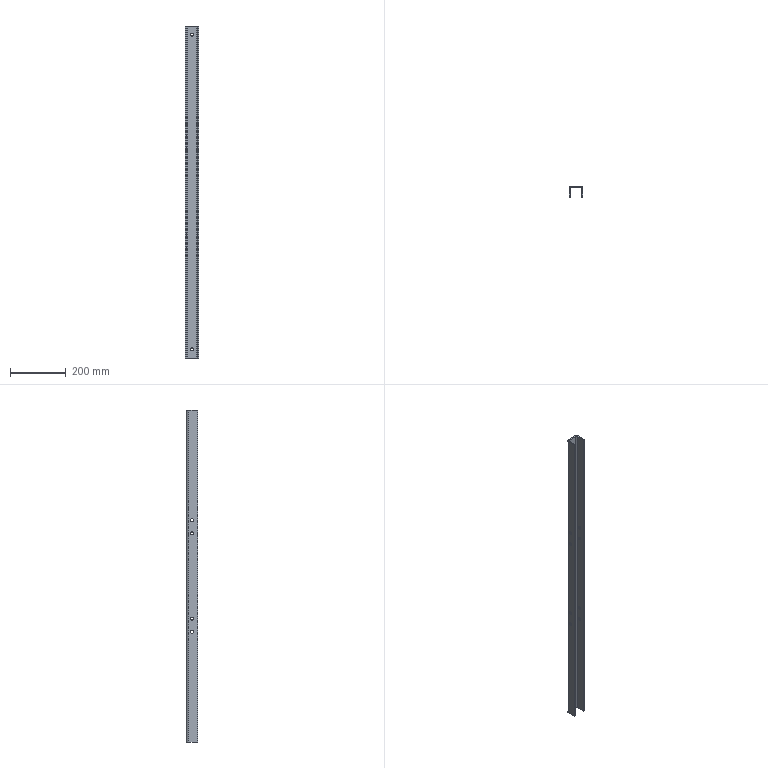Part | SolidWorks | features ICE 3, FlatPattern 1, SMBaseFlange 1, SheetMetal 1 | 1 solid | 42 faces | box 50 x 40 x 1190 mm | volume 552403 mm3 | cylinder 24 | plane 18 | commonest cylinder face diameters 11 x20 8 x2 16 x2
STEP:
#1=CARTESIAN_POINT('',(21.,-20.,205.5));
#2=VERTEX_POINT('',#1);
#3=CARTESIAN_POINT('',(21.,-20.,194.5));
#4=VERTEX_POINT('',#3);
#5=CARTESIAN_POINT('',(21.,-20.,200.));
#6=DIRECTION('',(1.,0.,0.));
#7=DIRECTION('',(0.,0.,-1.));
#8=AXIS2_PLACEMENT_3D('',#5,#6,#7);
#9=CIRCLE('',#8,5.5);
#10=EDGE_CURVE('',#2,#4,#9,.T.);
#11=ORIENTED_EDGE('',*,*,#10,.F.);
#12=CARTESIAN_POINT('',(25.,-20.,205.5));
#13=VERTEX_POINT('',#12);
#14=CARTESIAN_POINT('',(-25.,-20.,205.5));
#15=DIRECTION('',(1.,0.,0.));
#16=VECTOR('',#15,1000.);
#17=LINE('',#14,#16);
#18=EDGE_CURVE('',#2,#13,#17,.T.);
#19=ORIENTED_EDGE('',*,*,#18,.T.);
#20=CARTESIAN_POINT('',(25.,-20.,194.5));
#21=VERTEX_POINT('',#20);
#22=CARTESIAN_POINT('',(25.,-20.,200.));
#23=DIRECTION('',(1.,0.,0.));
#24=DIRECTION('',(0.,0.,-1.));
#25=AXIS2_PLACEMENT_3D('',#22,#23,#24);
#26=CIRCLE('',#25,5.5);
#27=EDGE_CURVE('',#13,#21,#26,.T.);
#28=ORIENTED_EDGE('',*,*,#27,.T.);
#29=CARTESIAN_POINT('',(-25.,-20.,194.5));
#30=DIRECTION('',(1.,0.,0.));
#31=VECTOR('',#30,1000.);
#32=LINE('',#29,#31);
#33=EDGE_CURVE('',#4,#21,#32,.T.);
#34=ORIENTED_EDGE('',*,*,#33,.F.);
#35=EDGE_LOOP('',(#11,#19,#28,#34));
#36=FACE_OUTER_BOUND('',#35,.T.);
#37=CARTESIAN_POINT('',(-25.,-20.,200.));
#38=DIRECTION('',(1.,0.,0.));
#39=DIRECTION('',(0.,0.,-1.));
#40=AXIS2_PLACEMENT_3D('',#37,#38,#39);
#41=CYLINDRICAL_SURFACE('',#40,5.5);
#42=ADVANCED_FACE('',(#36),#41,.F.);
#43=CARTESIAN_POINT('',(21.,-20.,158.));
#44=VERTEX_POINT('',#43);
#45=CARTESIAN_POINT('',(21.,-20.,147.));
#46=VERTEX_POINT('',#45);
#47=CARTESIAN_POINT('',(21.,-20.,152.5));
#48=DIRECTION('',(1.,0.,0.));
#49=DIRECTION('',(0.,0.,-1.));
#50=AXIS2_PLACEMENT_3D('',#47,#48,#49);
#51=CIRCLE('',#50,5.5);
#52=EDGE_CURVE('',#44,#46,#51,.T.);
#53=ORIENTED_EDGE('',*,*,#52,.F.);
#54=CARTESIAN_POINT('',(25.,-20.,158.));
#55=VERTEX_POINT('',#54);
#56=CARTESIAN_POINT('',(-25.,-20.,158.));
#57=DIRECTION('',(1.,0.,0.));
#58=VECTOR('',#57,1000.);
#59=LINE('',#56,#58);
#60=EDGE_CURVE('',#44,#55,#59,.T.);
#61=ORIENTED_EDGE('',*,*,#60,.T.);
#62=CARTESIAN_POINT('',(25.,-20.,147.));
#63=VERTEX_POINT('',#62);
#64=CARTESIAN_POINT('',(25.,-20.,152.5));
#65=DIRECTION('',(1.,0.,0.));
#66=DIRECTION('',(0.,0.,-1.));
#67=AXIS2_PLACEMENT_3D('',#64,#65,#66);
#68=CIRCLE('',#67,5.5);
#69=EDGE_CURVE('',#55,#63,#68,.T.);
#70=ORIENTED_EDGE('',*,*,#69,.T.);
#71=CARTESIAN_POINT('',(-25.,-20.,147.));
#72=DIRECTION('',(1.,0.,0.));
#73=VECTOR('',#72,1000.);
#74=LINE('',#71,#73);
#75=EDGE_CURVE('',#46,#63,#74,.T.);
#76=ORIENTED_EDGE('',*,*,#75,.F.);
#77=EDGE_LOOP('',(#53,#61,#70,#76));
#78=FACE_OUTER_BOUND('',#77,.T.);
#79=CARTESIAN_POINT('',(-25.,-20.,152.5));
#80=DIRECTION('',(1.,0.,0.));
#81=DIRECTION('',(0.,0.,-1.));
#82=AXIS2_PLACEMENT_3D('',#79,#80,#81);
#83=CYLINDRICAL_SURFACE('',#82,5.5);
#84=ADVANCED_FACE('',(#78),#83,.F.);
#85=CARTESIAN_POINT('',(21.,-20.,-147.));
#86=VERTEX_POINT('',#85);
#87=CARTESIAN_POINT('',(21.,-20.,-158.));
#88=VERTEX_POINT('',#87);
#89=CARTESIAN_POINT('',(21.,-20.,-152.5));
#90=DIRECTION('',(1.,0.,0.));
#91=DIRECTION('',(0.,0.,-1.));
#92=AXIS2_PLACEMENT_3D('',#89,#90,#91);
#93=CIRCLE('',#92,5.5);
#94=EDGE_CURVE('',#86,#88,#93,.T.);
#95=ORIENTED_EDGE('',*,*,#94,.F.);
#96=CARTESIAN_POINT('',(25.,-20.,-147.));
#97=VERTEX_POINT('',#96);
#98=CARTESIAN_POINT('',(-25.,-20.,-147.));
#99=DIRECTION('',(1.,0.,0.));
#100=VECTOR('',#99,1000.);
#101=LINE('',#98,#100);
#102=EDGE_CURVE('',#86,#97,#101,.T.);
#103=ORIENTED_EDGE('',*,*,#102,.T.);
#104=CARTESIAN_POINT('',(25.,-20.,-158.));
#105=VERTEX_POINT('',#104);
#106=CARTESIAN_POINT('',(25.,-20.,-152.5));
#107=DIRECTION('',(1.,0.,0.));
#108=DIRECTION('',(0.,0.,1.));
#109=AXIS2_PLACEMENT_3D('',#106,#107,#108);
#110=CIRCLE('',#109,5.5);
#111=EDGE_CURVE('',#97,#105,#110,.T.);
#112=ORIENTED_EDGE('',*,*,#111,.T.);
#113=CARTESIAN_POINT('',(-25.,-20.,-158.));
#114=DIRECTION('',(1.,0.,0.));
#115=VECTOR('',#114,1000.);
#116=LINE('',#113,#115);
#117=EDGE_CURVE('',#88,#105,#116,.T.);
#118=ORIENTED_EDGE('',*,*,#117,.F.);
#119=EDGE_LOOP('',(#95,#103,#112,#118));
#120=FACE_OUTER_BOUND('',#119,.T.);
#121=CARTESIAN_POINT('',(-25.,-20.,-152.5));
#122=DIRECTION('',(1.,0.,0.));
#123=DIRECTION('',(0.,0.,-1.));
#124=AXIS2_PLACEMENT_3D('',#121,#122,#123);
#125=CYLINDRICAL_SURFACE('',#124,5.5);
#126=ADVANCED_FACE('',(#120),#125,.F.);
#127=CARTESIAN_POINT('',(21.,-20.,-194.5));
#128=VERTEX_POINT('',#127);
#129=CARTESIAN_POINT('',(21.,-20.,-205.5));
#130=VERTEX_POINT('',#129);
#131=CARTESIAN_POINT('',(21.,-20.,-200.));
#132=DIRECTION('',(1.,0.,0.));
#133=DIRECTION('',(0.,0.,-1.));
#134=AXIS2_PLACEMENT_3D('',#131,#132,#133);
#135=CIRCLE('',#134,5.5);
#136=EDGE_CURVE('',#128,#130,#135,.T.);
#137=ORIENTED_EDGE('',*,*,#136,.F.);
#138=CARTESIAN_POINT('',(25.,-20.,-194.5));
#139=VERTEX_POINT('',#138);
#140=CARTESIAN_POINT('',(-25.,-20.,-194.5));
#141=DIRECTION('',(1.,0.,0.));
#142=VECTOR('',#141,1000.);
#143=LINE('',#140,#142);
#144=EDGE_CURVE('',#128,#139,#143,.T.);
#145=ORIENTED_EDGE('',*,*,#144,.T.);
#146=CARTESIAN_POINT('',(25.,-20.,-205.5));
#147=VERTEX_POINT('',#146);
#148=CARTESIAN_POINT('',(25.,-20.,-200.));
#149=DIRECTION('',(1.,0.,0.));
#150=DIRECTION('',(0.,0.,1.));
#151=AXIS2_PLACEMENT_3D('',#148,#149,#150);
#152=CIRCLE('',#151,5.5);
#153=EDGE_CURVE('',#139,#147,#152,.T.);
#154=ORIENTED_EDGE('',*,*,#153,.T.);
#155=CARTESIAN_POINT('',(-25.,-20.,-205.5));
#156=DIRECTION('',(1.,0.,0.));
#157=VECTOR('',#156,1000.);
#158=LINE('',#155,#157);
#159=EDGE_CURVE('',#130,#147,#158,.T.);
#160=ORIENTED_EDGE('',*,*,#159,.F.);
#161=EDGE_LOOP('',(#137,#145,#154,#160));
#162=FACE_OUTER_BOUND('',#161,.T.);
#163=CARTESIAN_POINT('',(-25.,-20.,-200.));
#164=DIRECTION('',(1.,0.,0.));
#165=DIRECTION('',(0.,0.,-1.));
#166=AXIS2_PLACEMENT_3D('',#163,#164,#165);
#167=CYLINDRICAL_SURFACE('',#166,5.5);
#168=ADVANCED_FACE('',(#162),#167,.F.);
#169=CARTESIAN_POINT('',(-25.,-20.,205.5));
#170=VERTEX_POINT('',#169);
#171=CARTESIAN_POINT('',(-25.,-20.,194.5));
#172=VERTEX_POINT('',#171);
#173=CARTESIAN_POINT('',(-25.,-20.,200.));
#174=DIRECTION('',(1.,0.,0.));
#175=DIRECTION('',(0.,0.,-1.));
#176=AXIS2_PLACEMENT_3D('',#173,#174,#175);
#177=CIRCLE('',#176,5.5);
#178=EDGE_CURVE('',#170,#172,#177,.T.);
#179=ORIENTED_EDGE('',*,*,#178,.F.);
#180=CARTESIAN_POINT('',(-21.,-20.,205.5));
#181=VERTEX_POINT('',#180);
#182=CARTESIAN_POINT('',(-25.,-20.,205.5));
#183=DIRECTION('',(1.,0.,0.));
#184=VECTOR('',#183,1000.);
#185=LINE('',#182,#184);
#186=EDGE_CURVE('',#170,#181,#185,.T.);
#187=ORIENTED_EDGE('',*,*,#186,.T.);
#188=CARTESIAN_POINT('',(-21.,-20.,194.5));
#189=VERTEX_POINT('',#188);
#190=CARTESIAN_POINT('',(-21.,-20.,200.));
#191=DIRECTION('',(-1.,0.,0.));
#192=DIRECTION('',(0.,0.,1.));
#193=AXIS2_PLACEMENT_3D('',#190,#191,#192);
#194=CIRCLE('',#193,5.5);
#195=EDGE_CURVE('',#189,#181,#194,.T.);
#196=ORIENTED_EDGE('',*,*,#195,.F.);
#197=CARTESIAN_POINT('',(-25.,-20.,194.5));
#198=DIRECTION('',(1.,0.,0.));
#199=VECTOR('',#198,1000.);
#200=LINE('',#197,#199);
#201=EDGE_CURVE('',#172,#189,#200,.T.);
#202=ORIENTED_EDGE('',*,*,#201,.F.);
#203=EDGE_LOOP('',(#179,#187,#196,#202));
#204=FACE_OUTER_BOUND('',#203,.T.);
#205=CARTESIAN_POINT('',(-25.,-20.,200.));
#206=DIRECTION('',(1.,0.,0.));
#207=DIRECTION('',(0.,0.,-1.));
#208=AXIS2_PLACEMENT_3D('',#205,#206,#207);
#209=CYLINDRICAL_SURFACE('',#208,5.5);
#210=ADVANCED_FACE('',(#204),#209,.F.);
#211=CARTESIAN_POINT('',(-25.,-20.,158.));
#212=VERTEX_POINT('',#211);
#213=CARTESIAN_POINT('',(-25.,-20.,147.));
#214=VERTEX_POINT('',#213);
#215=CARTESIAN_POINT('',(-25.,-20.,152.5));
#216=DIRECTION('',(1.,0.,0.));
#217=DIRECTION('',(0.,0.,-1.));
#218=AXIS2_PLACEMENT_3D('',#215,#216,#217);
#219=CIRCLE('',#218,5.5);
#220=EDGE_CURVE('',#212,#214,#219,.T.);
#221=ORIENTED_EDGE('',*,*,#220,.F.);
#222=CARTESIAN_POINT('',(-21.,-20.,158.));
#223=VERTEX_POINT('',#222);
#224=CARTESIAN_POINT('',(-25.,-20.,158.));
#225=DIRECTION('',(1.,0.,0.));
#226=VECTOR('',#225,1000.);
#227=LINE('',#224,#226);
#228=EDGE_CURVE('',#212,#223,#227,.T.);
#229=ORIENTED_EDGE('',*,*,#228,.T.);
#230=CARTESIAN_POINT('',(-21.,-20.,147.));
#231=VERTEX_POINT('',#230);
#232=CARTESIAN_POINT('',(-21.,-20.,152.5));
#233=DIRECTION('',(-1.,0.,0.));
#234=DIRECTION('',(0.,0.,1.));
#235=AXIS2_PLACEMENT_3D('',#232,#233,#234);
#236=CIRCLE('',#235,5.5);
#237=EDGE_CURVE('',#231,#223,#236,.T.);
#238=ORIENTED_EDGE('',*,*,#237,.F.);
#239=CARTESIAN_POINT('',(-25.,-20.,147.));
#240=DIRECTION('',(1.,0.,0.));
#241=VECTOR('',#240,1000.);
#242=LINE('',#239,#241);
#243=EDGE_CURVE('',#214,#231,#242,.T.);
#244=ORIENTED_EDGE('',*,*,#243,.F.);
#245=EDGE_LOOP('',(#221,#229,#238,#244));
#246=FACE_OUTER_BOUND('',#245,.T.);
#247=CARTESIAN_POINT('',(-25.,-20.,152.5));
#248=DIRECTION('',(1.,0.,0.));
#249=DIRECTION('',(0.,0.,-1.));
#250=AXIS2_PLACEMENT_3D('',#247,#248,#249);
#251=CYLINDRICAL_SURFACE('',#250,5.5);
#252=ADVANCED_FACE('',(#246),#251,.F.);
#253=CARTESIAN_POINT('',(-25.,-20.,-147.));
#254=VERTEX_POINT('',#253);
#255=CARTESIAN_POINT('',(-25.,-20.,-158.));
#256=VERTEX_POINT('',#255);
#257=CARTESIAN_POINT('',(-25.,-20.,-152.5));
#258=DIRECTION('',(1.,0.,0.));
#259=DIRECTION('',(0.,0.,1.));
#260=AXIS2_PLACEMENT_3D('',#257,#258,#259);
#261=CIRCLE('',#260,5.5);
#262=EDGE_CURVE('',#254,#256,#261,.T.);
#263=ORIENTED_EDGE('',*,*,#262,.F.);
#264=CARTESIAN_POINT('',(-21.,-20.,-147.));
#265=VERTEX_POINT('',#264);
#266=CARTESIAN_POINT('',(-25.,-20.,-147.));
#267=DIRECTION('',(1.,0.,0.));
#268=VECTOR('',#267,1000.);
#269=LINE('',#266,#268);
#270=EDGE_CURVE('',#254,#265,#269,.T.);
#271=ORIENTED_EDGE('',*,*,#270,.T.);
#272=CARTESIAN_POINT('',(-21.,-20.,-158.));
#273=VERTEX_POINT('',#272);
#274=CARTESIAN_POINT('',(-21.,-20.,-152.5));
#275=DIRECTION('',(-1.,0.,0.));
#276=DIRECTION('',(0.,0.,1.));
#277=AXIS2_PLACEMENT_3D('',#274,#275,#276);
#278=CIRCLE('',#277,5.5);
#279=EDGE_CURVE('',#273,#265,#278,.T.);
#280=ORIENTED_EDGE('',*,*,#279,.F.);
#281=CARTESIAN_POINT('',(-25.,-20.,-158.));
#282=DIRECTION('',(1.,0.,0.));
#283=VECTOR('',#282,1000.);
#284=LINE('',#281,#283);
#285=EDGE_CURVE('',#256,#273,#284,.T.);
#286=ORIENTED_EDGE('',*,*,#285,.F.);
#287=EDGE_LOOP('',(#263,#271,#280,#286));
#288=FACE_OUTER_BOUND('',#287,.T.);
#289=CARTESIAN_POINT('',(-25.,-20.,-152.5));
#290=DIRECTION('',(1.,0.,0.));
#291=DIRECTION('',(0.,0.,-1.));
#292=AXIS2_PLACEMENT_3D('',#289,#290,#291);
#293=CYLINDRICAL_SURFACE('',#292,5.5);
#294=ADVANCED_FACE('',(#288),#293,.F.);
#295=CARTESIAN_POINT('',(-25.,-20.,-194.5));
#296=VERTEX_POINT('',#295);
#297=CARTESIAN_POINT('',(-25.,-20.,-205.5));
#298=VERTEX_POINT('',#297);
#299=CARTESIAN_POINT('',(-25.,-20.,-200.));
#300=DIRECTION('',(1.,0.,0.));
#301=DIRECTION('',(0.,0.,1.));
#302=AXIS2_PLACEMENT_3D('',#299,#300,#301);
#303=CIRCLE('',#302,5.5);
#304=EDGE_CURVE('',#296,#298,#303,.T.);
#305=ORIENTED_EDGE('',*,*,#304,.F.);
#306=CARTESIAN_POINT('',(-21.,-20.,-194.5));
#307=VERTEX_POINT('',#306);
#308=CARTESIAN_POINT('',(-25.,-20.,-194.5));
#309=DIRECTION('',(1.,0.,0.));
#310=VECTOR('',#309,1000.);
#311=LINE('',#308,#310);
#312=EDGE_CURVE('',#296,#307,#311,.T.);
#313=ORIENTED_EDGE('',*,*,#312,.T.);
#314=CARTESIAN_POINT('',(-21.,-20.,-205.5));
#315=VERTEX_POINT('',#314);
#316=CARTESIAN_POINT('',(-21.,-20.,-200.));
#317=DIRECTION('',(-1.,0.,0.));
#318=DIRECTION('',(0.,0.,1.));
#319=AXIS2_PLACEMENT_3D('',#316,#317,#318);
#320=CIRCLE('',#319,5.5);
#321=EDGE_CURVE('',#315,#307,#320,.T.);
#322=ORIENTED_EDGE('',*,*,#321,.F.);
#323=CARTESIAN_POINT('',(-25.,-20.,-205.5));
#324=DIRECTION('',(1.,0.,0.));
#325=VECTOR('',#324,1000.);
#326=LINE('',#323,#325);
#327=EDGE_CURVE('',#298,#315,#326,.T.);
#328=ORIENTED_EDGE('',*,*,#327,.F.);
#329=EDGE_LOOP('',(#305,#313,#322,#328));
#330=FACE_OUTER_BOUND('',#329,.T.);
#331=CARTESIAN_POINT('',(-25.,-20.,-200.));
#332=DIRECTION('',(1.,0.,0.));
#333=DIRECTION('',(0.,0.,-1.));
#334=AXIS2_PLACEMENT_3D('',#331,#332,#333);
#335=CYLINDRICAL_SURFACE('',#334,5.5);
#336=ADVANCED_FACE('',(#330),#335,.F.);
#337=CARTESIAN_POINT('',(5.5,-4.,564.));
#338=VERTEX_POINT('',#337);
#339=CARTESIAN_POINT('',(-5.5,-4.,564.));
#340=VERTEX_POINT('',#339);
#341=CARTESIAN_POINT('',(0.,-4.,564.));
#342=DIRECTION('',(0.,1.,0.));
#343=DIRECTION('',(0.,0.,1.));
#344=AXIS2_PLACEMENT_3D('',#341,#342,#343);
#345=CIRCLE('',#344,5.5);
#346=EDGE_CURVE('',#338,#340,#345,.T.);
#347=ORIENTED_EDGE('',*,*,#346,.F.);
#348=CARTESIAN_POINT('',(5.5,0.,564.));
#349=VERTEX_POINT('',#348);
#350=CARTESIAN_POINT('',(5.5,-40.,564.));
#351=DIRECTION('',(0.,1.,0.));
#352=VECTOR('',#351,1000.);
#353=LINE('',#350,#352);
#354=EDGE_CURVE('',#338,#349,#353,.T.);
#355=ORIENTED_EDGE('',*,*,#354,.T.);
#356=CARTESIAN_POINT('',(-5.5,0.,564.));
#357=VERTEX_POINT('',#356);
#358=CARTESIAN_POINT('',(0.,0.,564.));
#359=DIRECTION('',(0.,1.,0.));
#360=DIRECTION('',(-1.,0.,0.));
#361=AXIS2_PLACEMENT_3D('',#358,#359,#360);
#362=CIRCLE('',#361,5.5);
#363=EDGE_CURVE('',#349,#357,#362,.T.);
#364=ORIENTED_EDGE('',*,*,#363,.T.);
#365=CARTESIAN_POINT('',(-5.5,-40.,564.));
#366=DIRECTION('',(0.,1.,0.));
#367=VECTOR('',#366,1000.);
#368=LINE('',#365,#367);
#369=EDGE_CURVE('',#340,#357,#368,.T.);
#370=ORIENTED_EDGE('',*,*,#369,.F.);
#371=EDGE_LOOP('',(#347,#355,#364,#370));
#372=FACE_OUTER_BOUND('',#371,.T.);
#373=CARTESIAN_POINT('',(0.,-40.,564.));
#374=DIRECTION('',(0.,1.,0.));
#375=DIRECTION('',(-1.,0.,0.));
#376=AXIS2_PLACEMENT_3D('',#373,#374,#375);
#377=CYLINDRICAL_SURFACE('',#376,5.5);
#378=ADVANCED_FACE('',(#372),#377,.F.);
#379=CARTESIAN_POINT('',(5.5,-4.,-564.));
#380=VERTEX_POINT('',#379);
#381=CARTESIAN_POINT('',(-5.5,-4.,-564.));
#382=VERTEX_POINT('',#381);
#383=CARTESIAN_POINT('',(0.,-4.,-564.));
#384=DIRECTION('',(0.,1.,0.));
#385=DIRECTION('',(0.,0.,1.));
#386=AXIS2_PLACEMENT_3D('',#383,#384,#385);
#387=CIRCLE('',#386,5.5);
#388=EDGE_CURVE('',#380,#382,#387,.T.);
#389=ORIENTED_EDGE('',*,*,#388,.F.);
#390=CARTESIAN_POINT('',(5.5,0.,-564.));
#391=VERTEX_POINT('',#390);
#392=CARTESIAN_POINT('',(5.5,-40.,-564.));
#393=DIRECTION('',(0.,1.,0.));
#394=VECTOR('',#393,1000.);
#395=LINE('',#392,#394);
#396=EDGE_CURVE('',#380,#391,#395,.T.);
#397=ORIENTED_EDGE('',*,*,#396,.T.);
#398=CARTESIAN_POINT('',(-5.5,0.,-564.));
#399=VERTEX_POINT('',#398);
#400=CARTESIAN_POINT('',(0.,0.,-564.));
#401=DIRECTION('',(0.,1.,0.));
#402=DIRECTION('',(1.,0.,0.));
#403=AXIS2_PLACEMENT_3D('',#400,#401,#402);
#404=CIRCLE('',#403,5.5);
#405=EDGE_CURVE('',#391,#399,#404,.T.);
#406=ORIENTED_EDGE('',*,*,#405,.T.);
#407=CARTESIAN_POINT('',(-5.5,-40.,-564.));
#408=DIRECTION('',(0.,1.,0.));
#409=VECTOR('',#408,1000.);
#410=LINE('',#407,#409);
#411=EDGE_CURVE('',#382,#399,#410,.T.);
#412=ORIENTED_EDGE('',*,*,#411,.F.);
#413=EDGE_LOOP('',(#389,#397,#406,#412));
#414=FACE_OUTER_BOUND('',#413,.T.);
#415=CARTESIAN_POINT('',(0.,-40.,-564.));
#416=DIRECTION('',(0.,1.,0.));
#417=DIRECTION('',(-1.,0.,0.));
#418=AXIS2_PLACEMENT_3D('',#415,#416,#417);
#419=CYLINDRICAL_SURFACE('',#418,5.5);
#420=ADVANCED_FACE('',(#414),#419,.F.);
#421=CARTESIAN_POINT('',(-17.,0.,595.));
#422=VERTEX_POINT('',#421);
#423=CARTESIAN_POINT('',(-17.,-4.,595.));
#424=VERTEX_POINT('',#423);
#425=CARTESIAN_POINT('',(-17.,0.,595.));
#426=DIRECTION('',(0.,-1.,0.));
#427=VECTOR('',#426,1000.);
#428=LINE('',#425,#427);
#429=EDGE_CURVE('',#422,#424,#428,.T.);
#430=ORIENTED_EDGE('',*,*,#429,.F.);
#431=CARTESIAN_POINT('',(-25.,-8.,595.));
#432=VERTEX_POINT('',#431);
#433=CARTESIAN_POINT('',(-17.,-8.,595.));
#434=DIRECTION('',(0.,0.,-1.));
#435=DIRECTION('',(1.,0.,0.));
#436=AXIS2_PLACEMENT_3D('',#433,#434,#435);
#437=CIRCLE('',#436,8.);
#438=EDGE_CURVE('',#432,#422,#437,.T.);
#439=ORIENTED_EDGE('',*,*,#438,.F.);
#440=CARTESIAN_POINT('',(-21.,-8.,595.));
#441=VERTEX_POINT('',#440);
#442=CARTESIAN_POINT('',(-21.,-8.,595.));
#443=DIRECTION('',(-1.,0.,0.));
#444=VECTOR('',#443,1000.);
#445=LINE('',#442,#444);
#446=EDGE_CURVE('',#441,#432,#445,.T.);
#447=ORIENTED_EDGE('',*,*,#446,.F.);
#448=CARTESIAN_POINT('',(-17.,-8.,595.));
#449=DIRECTION('',(0.,0.,-1.));
#450=DIRECTION('',(1.,0.,0.));
#451=AXIS2_PLACEMENT_3D('',#448,#449,#450);
#452=CIRCLE('',#451,4.);
#453=EDGE_CURVE('',#441,#424,#452,.T.);
#454=ORIENTED_EDGE('',*,*,#453,.T.);
#455=EDGE_LOOP('',(#430,#439,#447,#454));
#456=FACE_OUTER_BOUND('',#455,.T.);
#457=CARTESIAN_POINT('',(-17.,0.,595.));
#458=DIRECTION('',(0.,0.,1.));
#459=DIRECTION('',(1.,0.,0.));
#460=AXIS2_PLACEMENT_3D('',#457,#458,#459);
#461=PLANE('',#460);
#462=ADVANCED_FACE('',(#456),#461,.T.);
#463=CARTESIAN_POINT('',(17.,0.,595.));
#464=VERTEX_POINT('',#463);
#465=CARTESIAN_POINT('',(-25.,0.,595.));
#466=DIRECTION('',(1.,0.,0.));
#467=VECTOR('',#466,1000.);
#468=LINE('',#465,#467);
#469=EDGE_CURVE('',#422,#464,#468,.T.);
#470=ORIENTED_EDGE('',*,*,#469,.F.);
#471=ORIENTED_EDGE('',*,*,#429,.T.);
#472=CARTESIAN_POINT('',(17.,-4.,595.));
#473=VERTEX_POINT('',#472);
#474=CARTESIAN_POINT('',(-25.,-4.,595.));
#475=DIRECTION('',(1.,0.,0.));
#476=VECTOR('',#475,1000.);
#477=LINE('',#474,#476);
#478=EDGE_CURVE('',#424,#473,#477,.T.);
#479=ORIENTED_EDGE('',*,*,#478,.T.);
#480=CARTESIAN_POINT('',(17.,-4.,595.));
#481=DIRECTION('',(0.,1.,0.));
#482=VECTOR('',#481,1000.);
#483=LINE('',#480,#482);
#484=EDGE_CURVE('',#473,#464,#483,.T.);
#485=ORIENTED_EDGE('',*,*,#484,.T.);
#486=EDGE_LOOP('',(#470,#471,#479,#485));
#487=FACE_OUTER_BOUND('',#486,.T.);
#488=CARTESIAN_POINT('',(-21.,-8.,595.));
#489=DIRECTION('',(0.,0.,1.));
#490=DIRECTION('',(1.,0.,0.));
#491=AXIS2_PLACEMENT_3D('',#488,#489,#490);
#492=PLANE('',#491);
#493=ADVANCED_FACE('',(#487),#492,.T.);
#494=CARTESIAN_POINT('',(-25.,-8.,-595.));
#495=VERTEX_POINT('',#494);
#496=CARTESIAN_POINT('',(-21.,-8.,-595.));
#497=VERTEX_POINT('',#496);
#498=CARTESIAN_POINT('',(-25.,-8.,-595.));
#499=DIRECTION('',(1.,0.,0.));
#500=VECTOR('',#499,1000.);
#501=LINE('',#498,#500);
#502=EDGE_CURVE('',#495,#497,#501,.T.);
#503=ORIENTED_EDGE('',*,*,#502,.F.);
#504=CARTESIAN_POINT('',(-17.,0.,-595.));
#505=VERTEX_POINT('',#504);
#506=CARTESIAN_POINT('',(-17.,-8.,-595.));
#507=DIRECTION('',(0.,0.,-1.));
#508=DIRECTION('',(1.,0.,0.));
#509=AXIS2_PLACEMENT_3D('',#506,#507,#508);
#510=CIRCLE('',#509,8.);
#511=EDGE_CURVE('',#495,#505,#510,.T.);
#512=ORIENTED_EDGE('',*,*,#511,.T.);
#513=CARTESIAN_POINT('',(-17.,-4.,-595.));
#514=VERTEX_POINT('',#513);
#515=CARTESIAN_POINT('',(-17.,-4.,-595.));
#516=DIRECTION('',(0.,1.,0.));
#517=VECTOR('',#516,1000.);
#518=LINE('',#515,#517);
#519=EDGE_CURVE('',#514,#505,#518,.T.);
#520=ORIENTED_EDGE('',*,*,#519,.F.);
#521=CARTESIAN_POINT('',(-17.,-8.,-595.));
#522=DIRECTION('',(0.,0.,-1.));
#523=DIRECTION('',(1.,0.,0.));
#524=AXIS2_PLACEMENT_3D('',#521,#522,#523);
#525=CIRCLE('',#524,4.);
#526=EDGE_CURVE('',#497,#514,#525,.T.);
#527=ORIENTED_EDGE('',*,*,#526,.F.);
#528=EDGE_LOOP('',(#503,#512,#520,#527));
#529=FACE_OUTER_BOUND('',#528,.T.);
#530=CARTESIAN_POINT('',(-25.,-8.,-595.));
#531=DIRECTION('',(0.,0.,-1.));
#532=DIRECTION('',(-1.,0.,0.));
#533=AXIS2_PLACEMENT_3D('',#530,#531,#532);
#534=PLANE('',#533);
#535=ADVANCED_FACE('',(#529),#534,.T.);
#536=CARTESIAN_POINT('',(-25.,-40.,-595.));
#537=VERTEX_POINT('',#536);
#538=CARTESIAN_POINT('',(-25.,-40.,-595.));
#539=DIRECTION('',(0.,1.,0.));
#540=VECTOR('',#539,1000.);
#541=LINE('',#538,#540);
#542=EDGE_CURVE('',#537,#495,#541,.T.);
#543=ORIENTED_EDGE('',*,*,#542,.T.);
#544=ORIENTED_EDGE('',*,*,#502,.T.);
#545=CARTESIAN_POINT('',(-21.,-40.,-595.));
#546=VERTEX_POINT('',#545);
#547=CARTESIAN_POINT('',(-21.,-40.,-595.));
#548=DIRECTION('',(0.,1.,0.));
#549=VECTOR('',#548,1000.);
#550=LINE('',#547,#549);
#551=EDGE_CURVE('',#546,#497,#550,.T.);
#552=ORIENTED_EDGE('',*,*,#551,.F.);
#553=CARTESIAN_POINT('',(-21.,-40.,-595.));
#554=DIRECTION('',(-1.,0.,0.));
#555=VECTOR('',#554,1000.);
#556=LINE('',#553,#555);
#557=EDGE_CURVE('',#546,#537,#556,.T.);
#558=ORIENTED_EDGE('',*,*,#557,.T.);
#559=EDGE_LOOP('',(#543,#544,#552,#558));
#560=FACE_OUTER_BOUND('',#559,.T.);
#561=CARTESIAN_POINT('',(-17.,-4.,-595.));
#562=DIRECTION('',(0.,0.,-1.));
#563=DIRECTION('',(-1.,0.,0.));
#564=AXIS2_PLACEMENT_3D('',#561,#562,#563);
#565=PLANE('',#564);
#566=ADVANCED_FACE('',(#560),#565,.T.);
#567=CARTESIAN_POINT('',(25.,-8.,595.));
#568=VERTEX_POINT('',#567);
#569=CARTESIAN_POINT('',(21.,-8.,595.));
#570=VERTEX_POINT('',#569);
#571=CARTESIAN_POINT('',(25.,-8.,595.));
#572=DIRECTION('',(-1.,0.,0.));
#573=VECTOR('',#572,1000.);
#574=LINE('',#571,#573);
#575=EDGE_CURVE('',#568,#570,#574,.T.);
#576=ORIENTED_EDGE('',*,*,#575,.F.);
#577=CARTESIAN_POINT('',(17.,-8.,595.));
#578=DIRECTION('',(0.,0.,-1.));
#579=DIRECTION('',(1.,0.,0.));
#580=AXIS2_PLACEMENT_3D('',#577,#578,#579);
#581=CIRCLE('',#580,8.);
#582=EDGE_CURVE('',#464,#568,#581,.T.);
#583=ORIENTED_EDGE('',*,*,#582,.F.);
#584=ORIENTED_EDGE('',*,*,#484,.F.);
#585=CARTESIAN_POINT('',(17.,-8.,595.));
#586=DIRECTION('',(0.,0.,-1.));
#587=DIRECTION('',(1.,0.,0.));
#588=AXIS2_PLACEMENT_3D('',#585,#586,#587);
#589=CIRCLE('',#588,4.);
#590=EDGE_CURVE('',#473,#570,#589,.T.);
#591=ORIENTED_EDGE('',*,*,#590,.T.);
#592=EDGE_LOOP('',(#576,#583,#584,#591));
#593=FACE_OUTER_BOUND('',#592,.T.);
#594=CARTESIAN_POINT('',(25.,-8.,595.));
#595=DIRECTION('',(0.,0.,1.));
#596=DIRECTION('',(1.,0.,0.));
#597=AXIS2_PLACEMENT_3D('',#594,#595,#596);
#598=PLANE('',#597);
#599=ADVANCED_FACE('',(#593),#598,.T.);
#600=CARTESIAN_POINT('',(25.,-40.,595.));
#601=VERTEX_POINT('',#600);
#602=CARTESIAN_POINT('',(25.,0.,595.));
#603=DIRECTION('',(0.,-1.,0.));
#604=VECTOR('',#603,1000.);
#605=LINE('',#602,#604);
#606=EDGE_CURVE('',#568,#601,#605,.T.);
#607=ORIENTED_EDGE('',*,*,#606,.F.);
#608=ORIENTED_EDGE('',*,*,#575,.T.);
#609=CARTESIAN_POINT('',(21.,-40.,595.));
#610=VERTEX_POINT('',#609);
#611=CARTESIAN_POINT('',(21.,0.,595.));
#612=DIRECTION('',(0.,-1.,0.));
#613=VECTOR('',#612,1000.);
#614=LINE('',#611,#613);
#615=EDGE_CURVE('',#570,#610,#614,.T.);
#616=ORIENTED_EDGE('',*,*,#615,.T.);
#617=CARTESIAN_POINT('',(25.,-40.,595.));
#618=DIRECTION('',(-1.,0.,0.));
#619=VECTOR('',#618,1000.);
#620=LINE('',#617,#619);
#621=EDGE_CURVE('',#601,#610,#620,.T.);
#622=ORIENTED_EDGE('',*,*,#621,.F.);
#623=EDGE_LOOP('',(#607,#608,#616,#622));
#624=FACE_OUTER_BOUND('',#623,.T.);
#625=CARTESIAN_POINT('',(17.,-4.,595.));
#626=DIRECTION('',(0.,0.,1.));
#627=DIRECTION('',(1.,0.,0.));
#628=AXIS2_PLACEMENT_3D('',#625,#626,#627);
#629=PLANE('',#628);
#630=ADVANCED_FACE('',(#624),#629,.T.);
#631=CARTESIAN_POINT('',(17.,0.,-595.));
#632=VERTEX_POINT('',#631);
#633=CARTESIAN_POINT('',(17.,-4.,-595.));
#634=VERTEX_POINT('',#633);
#635=CARTESIAN_POINT('',(17.,0.,-595.));
#636=DIRECTION('',(0.,-1.,0.));
#637=VECTOR('',#636,1000.);
#638=LINE('',#635,#637);
#639=EDGE_CURVE('',#632,#634,#638,.T.);
#640=ORIENTED_EDGE('',*,*,#639,.F.);
#641=CARTESIAN_POINT('',(25.,-8.,-595.));
#642=VERTEX_POINT('',#641);
#643=CARTESIAN_POINT('',(17.,-8.,-595.));
#644=DIRECTION('',(0.,0.,-1.));
#645=DIRECTION('',(1.,0.,0.));
#646=AXIS2_PLACEMENT_3D('',#643,#644,#645);
#647=CIRCLE('',#646,8.);
#648=EDGE_CURVE('',#632,#642,#647,.T.);
#649=ORIENTED_EDGE('',*,*,#648,.T.);
#650=CARTESIAN_POINT('',(21.,-8.,-595.));
#651=VERTEX_POINT('',#650);
#652=CARTESIAN_POINT('',(21.,-8.,-595.));
#653=DIRECTION('',(1.,0.,0.));
#654=VECTOR('',#653,1000.);
#655=LINE('',#652,#654);
#656=EDGE_CURVE('',#651,#642,#655,.T.);
#657=ORIENTED_EDGE('',*,*,#656,.F.);
#658=CARTESIAN_POINT('',(17.,-8.,-595.));
#659=DIRECTION('',(0.,0.,-1.));
#660=DIRECTION('',(1.,0.,0.));
#661=AXIS2_PLACEMENT_3D('',#658,#659,#660);
#662=CIRCLE('',#661,4.);
#663=EDGE_CURVE('',#634,#651,#662,.T.);
#664=ORIENTED_EDGE('',*,*,#663,.F.);
#665=EDGE_LOOP('',(#640,#649,#657,#664));
#666=FACE_OUTER_BOUND('',#665,.T.);
#667=CARTESIAN_POINT('',(17.,0.,-595.));
#668=DIRECTION('',(0.,0.,-1.));
#669=DIRECTION('',(-1.,0.,0.));
#670=AXIS2_PLACEMENT_3D('',#667,#668,#669);
#671=PLANE('',#670);
#672=ADVANCED_FACE('',(#666),#671,.T.);
#673=CARTESIAN_POINT('',(-25.,0.,-595.));
#674=DIRECTION('',(1.,0.,0.));
#675=VECTOR('',#674,1000.);
#676=LINE('',#673,#675);
#677=EDGE_CURVE('',#505,#632,#676,.T.);
#678=ORIENTED_EDGE('',*,*,#677,.T.);
#679=ORIENTED_EDGE('',*,*,#639,.T.);
#680=CARTESIAN_POINT('',(-25.,-4.,-595.));
#681=DIRECTION('',(1.,0.,0.));
#682=VECTOR('',#681,1000.);
#683=LINE('',#680,#682);
#684=EDGE_CURVE('',#514,#634,#683,.T.);
#685=ORIENTED_EDGE('',*,*,#684,.F.);
#686=ORIENTED_EDGE('',*,*,#519,.T.);
#687=EDGE_LOOP('',(#678,#679,#685,#686));
#688=FACE_OUTER_BOUND('',#687,.T.);
#689=CARTESIAN_POINT('',(21.,-8.,-595.));
#690=DIRECTION('',(0.,0.,-1.));
#691=DIRECTION('',(-1.,0.,0.));
#692=AXIS2_PLACEMENT_3D('',#689,#690,#691);
#693=PLANE('',#692);
#694=ADVANCED_FACE('',(#688),#693,.T.);
#695=CARTESIAN_POINT('',(21.,-20.,200.));
#696=DIRECTION('',(1.,0.,0.));
#697=DIRECTION('',(0.,0.,-1.));
#698=AXIS2_PLACEMENT_3D('',#695,#696,#697);
#699=CIRCLE('',#698,5.5);
#700=EDGE_CURVE('',#4,#2,#699,.T.);
#701=ORIENTED_EDGE('',*,*,#700,.T.);
#702=ORIENTED_EDGE('',*,*,#10,.T.);
#703=EDGE_LOOP('',(#701,#702));
#704=FACE_BOUND('',#703,.T.);
#705=CARTESIAN_POINT('',(21.,-20.,152.5));
#706=DIRECTION('',(1.,0.,0.));
#707=DIRECTION('',(0.,0.,-1.));
#708=AXIS2_PLACEMENT_3D('',#705,#706,#707);
#709=CIRCLE('',#708,5.5);
#710=EDGE_CURVE('',#46,#44,#709,.T.);
#711=ORIENTED_EDGE('',*,*,#710,.T.);
#712=ORIENTED_EDGE('',*,*,#52,.T.);
#713=EDGE_LOOP('',(#711,#712));
#714=FACE_BOUND('',#713,.T.);
#715=CARTESIAN_POINT('',(21.,-20.,-152.5));
#716=DIRECTION('',(1.,0.,0.));
#717=DIRECTION('',(0.,0.,-1.));
#718=AXIS2_PLACEMENT_3D('',#715,#716,#717);
#719=CIRCLE('',#718,5.5);
#720=EDGE_CURVE('',#88,#86,#719,.T.);
#721=ORIENTED_EDGE('',*,*,#720,.T.);
#722=ORIENTED_EDGE('',*,*,#94,.T.);
#723=EDGE_LOOP('',(#721,#722));
#724=FACE_BOUND('',#723,.T.);
#725=CARTESIAN_POINT('',(21.,-20.,-200.));
#726=DIRECTION('',(1.,0.,0.));
#727=DIRECTION('',(0.,0.,-1.));
#728=AXIS2_PLACEMENT_3D('',#725,#726,#727);
#729=CIRCLE('',#728,5.5);
#730=EDGE_CURVE('',#130,#128,#729,.T.);
#731=ORIENTED_EDGE('',*,*,#730,.T.);
#732=ORIENTED_EDGE('',*,*,#136,.T.);
#733=EDGE_LOOP('',(#731,#732));
#734=FACE_BOUND('',#733,.T.);
#735=CARTESIAN_POINT('',(21.,-40.,-595.));
#736=VERTEX_POINT('',#735);
#737=CARTESIAN_POINT('',(21.,0.,-595.));
#738=DIRECTION('',(0.,-1.,0.));
#739=VECTOR('',#738,1000.);
#740=LINE('',#737,#739);
#741=EDGE_CURVE('',#651,#736,#740,.T.);
#742=ORIENTED_EDGE('',*,*,#741,.T.);
#743=CARTESIAN_POINT('',(21.,-40.,595.));
#744=DIRECTION('',(0.,0.,-1.));
#745=VECTOR('',#744,1000.);
#746=LINE('',#743,#745);
#747=EDGE_CURVE('',#610,#736,#746,.T.);
#748=ORIENTED_EDGE('',*,*,#747,.F.);
#749=ORIENTED_EDGE('',*,*,#615,.F.);
#750=CARTESIAN_POINT('',(21.,-8.,595.));
#751=DIRECTION('',(0.,0.,-1.));
#752=VECTOR('',#751,1000.);
#753=LINE('',#750,#752);
#754=EDGE_CURVE('',#570,#651,#753,.T.);
#755=ORIENTED_EDGE('',*,*,#754,.T.);
#756=EDGE_LOOP('',(#742,#748,#749,#755));
#757=FACE_OUTER_BOUND('',#756,.T.);
#758=CARTESIAN_POINT('',(21.,0.,595.));
#759=DIRECTION('',(1.,0.,0.));
#760=DIRECTION('',(0.,0.,-1.));
#761=AXIS2_PLACEMENT_3D('',#758,#759,#760);
#762=PLANE('',#761);
#763=ADVANCED_FACE('',(#704,#714,#724,#734,#757),#762,.F.);
#764=CARTESIAN_POINT('',(25.,-40.,-595.));
#765=VERTEX_POINT('',#764);
#766=CARTESIAN_POINT('',(25.,-40.,-595.));
#767=DIRECTION('',(-1.,0.,0.));
#768=VECTOR('',#767,1000.);
#769=LINE('',#766,#768);
#770=EDGE_CURVE('',#765,#736,#769,.T.);
#771=ORIENTED_EDGE('',*,*,#770,.F.);
#772=CARTESIAN_POINT('',(25.,-40.,595.));
#773=DIRECTION('',(0.,0.,-1.));
#774=VECTOR('',#773,1000.);
#775=LINE('',#772,#774);
#776=EDGE_CURVE('',#601,#765,#775,.T.);
#777=ORIENTED_EDGE('',*,*,#776,.F.);
#778=ORIENTED_EDGE('',*,*,#621,.T.);
#779=ORIENTED_EDGE('',*,*,#747,.T.);
#780=EDGE_LOOP('',(#771,#777,#778,#779));
#781=FACE_OUTER_BOUND('',#780,.T.);
#782=CARTESIAN_POINT('',(25.,-40.,595.));
#783=DIRECTION('',(0.,-1.,0.));
#784=DIRECTION('',(0.,0.,-1.));
#785=AXIS2_PLACEMENT_3D('',#782,#783,#784);
#786=PLANE('',#785);
#787=ADVANCED_FACE('',(#781),#786,.T.);
#788=CARTESIAN_POINT('',(25.,-20.,200.));
#789=DIRECTION('',(1.,0.,0.));
#790=DIRECTION('',(0.,0.,-1.));
#791=AXIS2_PLACEMENT_3D('',#788,#789,#790);
#792=CIRCLE('',#791,5.5);
#793=EDGE_CURVE('',#21,#13,#792,.T.);
#794=ORIENTED_EDGE('',*,*,#793,.F.);
#795=ORIENTED_EDGE('',*,*,#27,.F.);
#796=EDGE_LOOP('',(#794,#795));
#797=FACE_BOUND('',#796,.T.);
#798=CARTESIAN_POINT('',(25.,-20.,152.5));
#799=DIRECTION('',(1.,0.,0.));
#800=DIRECTION('',(0.,0.,-1.));
#801=AXIS2_PLACEMENT_3D('',#798,#799,#800);
#802=CIRCLE('',#801,5.5);
#803=EDGE_CURVE('',#63,#55,#802,.T.);
#804=ORIENTED_EDGE('',*,*,#803,.F.);
#805=ORIENTED_EDGE('',*,*,#69,.F.);
#806=EDGE_LOOP('',(#804,#805));
#807=FACE_BOUND('',#806,.T.);
#808=CARTESIAN_POINT('',(25.,-20.,-152.5));
#809=DIRECTION('',(1.,0.,0.));
#810=DIRECTION('',(0.,0.,1.));
#811=AXIS2_PLACEMENT_3D('',#808,#809,#810);
#812=CIRCLE('',#811,5.5);
#813=EDGE_CURVE('',#105,#97,#812,.T.);
#814=ORIENTED_EDGE('',*,*,#813,.F.);
#815=ORIENTED_EDGE('',*,*,#111,.F.);
#816=EDGE_LOOP('',(#814,#815));
#817=FACE_BOUND('',#816,.T.);
#818=CARTESIAN_POINT('',(25.,-20.,-200.));
#819=DIRECTION('',(1.,0.,0.));
#820=DIRECTION('',(0.,0.,1.));
#821=AXIS2_PLACEMENT_3D('',#818,#819,#820);
#822=CIRCLE('',#821,5.5);
#823=EDGE_CURVE('',#147,#139,#822,.T.);
#824=ORIENTED_EDGE('',*,*,#823,.F.);
#825=ORIENTED_EDGE('',*,*,#153,.F.);
#826=EDGE_LOOP('',(#824,#825));
#827=FACE_BOUND('',#826,.T.);
#828=CARTESIAN_POINT('',(25.,0.,-595.));
#829=DIRECTION('',(0.,-1.,0.));
#830=VECTOR('',#829,1000.);
#831=LINE('',#828,#830);
#832=EDGE_CURVE('',#642,#765,#831,.T.);
#833=ORIENTED_EDGE('',*,*,#832,.F.);
#834=CARTESIAN_POINT('',(25.,-8.,595.));
#835=DIRECTION('',(0.,0.,-1.));
#836=VECTOR('',#835,1000.);
#837=LINE('',#834,#836);
#838=EDGE_CURVE('',#568,#642,#837,.T.);
#839=ORIENTED_EDGE('',*,*,#838,.F.);
#840=ORIENTED_EDGE('',*,*,#606,.T.);
#841=ORIENTED_EDGE('',*,*,#776,.T.);
#842=EDGE_LOOP('',(#833,#839,#840,#841));
#843=FACE_OUTER_BOUND('',#842,.T.);
#844=CARTESIAN_POINT('',(25.,0.,595.));
#845=DIRECTION('',(1.,0.,0.));
#846=DIRECTION('',(0.,0.,-1.));
#847=AXIS2_PLACEMENT_3D('',#844,#845,#846);
#848=PLANE('',#847);
#849=ADVANCED_FACE('',(#797,#807,#817,#827,#843),#848,.T.);
#850=ORIENTED_EDGE('',*,*,#648,.F.);
#851=CARTESIAN_POINT('',(17.,0.,595.));
#852=DIRECTION('',(0.,0.,-1.));
#853=VECTOR('',#852,1000.);
#854=LINE('',#851,#853);
#855=EDGE_CURVE('',#464,#632,#854,.T.);
#856=ORIENTED_EDGE('',*,*,#855,.F.);
#857=ORIENTED_EDGE('',*,*,#582,.T.);
#858=ORIENTED_EDGE('',*,*,#838,.T.);
#859=EDGE_LOOP('',(#850,#856,#857,#858));
#860=FACE_OUTER_BOUND('',#859,.T.);
#861=CARTESIAN_POINT('',(17.,-8.,595.));
#862=DIRECTION('',(0.,0.,-1.));
#863=DIRECTION('',(-1.,0.,0.));
#864=AXIS2_PLACEMENT_3D('',#861,#862,#863);
#865=CYLINDRICAL_SURFACE('',#864,8.);
#866=ADVANCED_FACE('',(#860),#865,.T.);
#867=CARTESIAN_POINT('',(0.,0.,564.));
#868=DIRECTION('',(0.,1.,0.));
#869=DIRECTION('',(-1.,0.,0.));
#870=AXIS2_PLACEMENT_3D('',#867,#868,#869);
#871=CIRCLE('',#870,5.5);
#872=EDGE_CURVE('',#357,#349,#871,.T.);
#873=ORIENTED_EDGE('',*,*,#872,.F.);
#874=ORIENTED_EDGE('',*,*,#363,.F.);
#875=EDGE_LOOP('',(#873,#874));
#876=FACE_BOUND('',#875,.T.);
#877=CARTESIAN_POINT('',(0.,0.,-564.));
#878=DIRECTION('',(0.,1.,0.));
#879=DIRECTION('',(1.,0.,0.));
#880=AXIS2_PLACEMENT_3D('',#877,#878,#879);
#881=CIRCLE('',#880,5.5);
#882=EDGE_CURVE('',#399,#391,#881,.T.);
#883=ORIENTED_EDGE('',*,*,#882,.F.);
#884=ORIENTED_EDGE('',*,*,#405,.F.);
#885=EDGE_LOOP('',(#883,#884));
#886=FACE_BOUND('',#885,.T.);
#887=ORIENTED_EDGE('',*,*,#677,.F.);
#888=CARTESIAN_POINT('',(-17.,0.,595.));
#889=DIRECTION('',(0.,0.,-1.));
#890=VECTOR('',#889,1000.);
#891=LINE('',#888,#890);
#892=EDGE_CURVE('',#422,#505,#891,.T.);
#893=ORIENTED_EDGE('',*,*,#892,.F.);
#894=ORIENTED_EDGE('',*,*,#469,.T.);
#895=ORIENTED_EDGE('',*,*,#855,.T.);
#896=EDGE_LOOP('',(#887,#893,#894,#895));
#897=FACE_OUTER_BOUND('',#896,.T.);
#898=CARTESIAN_POINT('',(-25.,0.,595.));
#899=DIRECTION('',(0.,1.,0.));
#900=DIRECTION('',(0.,0.,1.));
#901=AXIS2_PLACEMENT_3D('',#898,#899,#900);
#902=PLANE('',#901);
#903=ADVANCED_FACE('',(#876,#886,#897),#902,.T.);
#904=ORIENTED_EDGE('',*,*,#511,.F.);
#905=CARTESIAN_POINT('',(-25.,-8.,595.));
#906=DIRECTION('',(0.,0.,-1.));
#907=VECTOR('',#906,1000.);
#908=LINE('',#905,#907);
#909=EDGE_CURVE('',#432,#495,#908,.T.);
#910=ORIENTED_EDGE('',*,*,#909,.F.);
#911=ORIENTED_EDGE('',*,*,#438,.T.);
#912=ORIENTED_EDGE('',*,*,#892,.T.);
#913=EDGE_LOOP('',(#904,#910,#911,#912));
#914=FACE_OUTER_BOUND('',#913,.T.);
#915=CARTESIAN_POINT('',(-17.,-8.,595.));
#916=DIRECTION('',(0.,0.,-1.));
#917=DIRECTION('',(-1.,0.,0.));
#918=AXIS2_PLACEMENT_3D('',#915,#916,#917);
#919=CYLINDRICAL_SURFACE('',#918,8.);
#920=ADVANCED_FACE('',(#914),#919,.T.);
#921=CARTESIAN_POINT('',(-25.,-20.,200.));
#922=DIRECTION('',(1.,0.,0.));
#923=DIRECTION('',(0.,0.,-1.));
#924=AXIS2_PLACEMENT_3D('',#921,#922,#923);
#925=CIRCLE('',#924,5.5);
#926=EDGE_CURVE('',#172,#170,#925,.T.);
#927=ORIENTED_EDGE('',*,*,#926,.T.);
#928=ORIENTED_EDGE('',*,*,#178,.T.);
#929=EDGE_LOOP('',(#927,#928));
#930=FACE_BOUND('',#929,.T.);
#931=CARTESIAN_POINT('',(-25.,-20.,152.5));
#932=DIRECTION('',(1.,0.,0.));
#933=DIRECTION('',(0.,0.,-1.));
#934=AXIS2_PLACEMENT_3D('',#931,#932,#933);
#935=CIRCLE('',#934,5.5);
#936=EDGE_CURVE('',#214,#212,#935,.T.);
#937=ORIENTED_EDGE('',*,*,#936,.T.);
#938=ORIENTED_EDGE('',*,*,#220,.T.);
#939=EDGE_LOOP('',(#937,#938));
#940=FACE_BOUND('',#939,.T.);
#941=CARTESIAN_POINT('',(-25.,-20.,-152.5));
#942=DIRECTION('',(1.,0.,0.));
#943=DIRECTION('',(0.,0.,1.));
#944=AXIS2_PLACEMENT_3D('',#941,#942,#943);
#945=CIRCLE('',#944,5.5);
#946=EDGE_CURVE('',#256,#254,#945,.T.);
#947=ORIENTED_EDGE('',*,*,#946,.T.);
#948=ORIENTED_EDGE('',*,*,#262,.T.);
#949=EDGE_LOOP('',(#947,#948));
#950=FACE_BOUND('',#949,.T.);
#951=CARTESIAN_POINT('',(-25.,-20.,-200.));
#952=DIRECTION('',(1.,0.,0.));
#953=DIRECTION('',(0.,0.,1.));
#954=AXIS2_PLACEMENT_3D('',#951,#952,#953);
#955=CIRCLE('',#954,5.5);
#956=EDGE_CURVE('',#298,#296,#955,.T.);
#957=ORIENTED_EDGE('',*,*,#956,.T.);
#958=ORIENTED_EDGE('',*,*,#304,.T.);
#959=EDGE_LOOP('',(#957,#958));
#960=FACE_BOUND('',#959,.T.);
#961=ORIENTED_EDGE('',*,*,#542,.F.);
#962=CARTESIAN_POINT('',(-25.,-40.,595.));
#963=VERTEX_POINT('',#962);
#964=CARTESIAN_POINT('',(-25.,-40.,595.));
#965=DIRECTION('',(0.,0.,-1.));
#966=VECTOR('',#965,1000.);
#967=LINE('',#964,#966);
#968=EDGE_CURVE('',#963,#537,#967,.T.);
#969=ORIENTED_EDGE('',*,*,#968,.F.);
#970=CARTESIAN_POINT('',(-25.,-40.,595.));
#971=DIRECTION('',(0.,1.,0.));
#972=VECTOR('',#971,1000.);
#973=LINE('',#970,#972);
#974=EDGE_CURVE('',#963,#432,#973,.T.);
#975=ORIENTED_EDGE('',*,*,#974,.T.);
#976=ORIENTED_EDGE('',*,*,#909,.T.);
#977=EDGE_LOOP('',(#961,#969,#975,#976));
#978=FACE_OUTER_BOUND('',#977,.T.);
#979=CARTESIAN_POINT('',(-25.,-40.,595.));
#980=DIRECTION('',(-1.,0.,0.));
#981=DIRECTION('',(0.,0.,1.));
#982=AXIS2_PLACEMENT_3D('',#979,#980,#981);
#983=PLANE('',#982);
#984=ADVANCED_FACE('',(#930,#940,#950,#960,#978),#983,.T.);
#985=ORIENTED_EDGE('',*,*,#557,.F.);
#986=CARTESIAN_POINT('',(-21.,-40.,595.));
#987=VERTEX_POINT('',#986);
#988=CARTESIAN_POINT('',(-21.,-40.,595.));
#989=DIRECTION('',(0.,0.,-1.));
#990=VECTOR('',#989,1000.);
#991=LINE('',#988,#990);
#992=EDGE_CURVE('',#987,#546,#991,.T.);
#993=ORIENTED_EDGE('',*,*,#992,.F.);
#994=CARTESIAN_POINT('',(-21.,-40.,595.));
#995=DIRECTION('',(-1.,0.,0.));
#996=VECTOR('',#995,1000.);
#997=LINE('',#994,#996);
#998=EDGE_CURVE('',#987,#963,#997,.T.);
#999=ORIENTED_EDGE('',*,*,#998,.T.);
#1000=ORIENTED_EDGE('',*,*,#968,.T.);
#1001=EDGE_LOOP('',(#985,#993,#999,#1000));
#1002=FACE_OUTER_BOUND('',#1001,.T.);
#1003=CARTESIAN_POINT('',(-21.,-40.,595.));
#1004=DIRECTION('',(0.,-1.,0.));
#1005=DIRECTION('',(0.,0.,-1.));
#1006=AXIS2_PLACEMENT_3D('',#1003,#1004,#1005);
#1007=PLANE('',#1006);
#1008=ADVANCED_FACE('',(#1002),#1007,.T.);
#1009=ORIENTED_EDGE('',*,*,#195,.T.);
#1010=CARTESIAN_POINT('',(-21.,-20.,200.));
#1011=DIRECTION('',(-1.,0.,0.));
#1012=DIRECTION('',(0.,0.,1.));
#1013=AXIS2_PLACEMENT_3D('',#1010,#1011,#1012);
#1014=CIRCLE('',#1013,5.5);
#1015=EDGE_CURVE('',#181,#189,#1014,.T.);
#1016=ORIENTED_EDGE('',*,*,#1015,.T.);
#1017=EDGE_LOOP('',(#1009,#1016));
#1018=FACE_BOUND('',#1017,.T.);
#1019=ORIENTED_EDGE('',*,*,#237,.T.);
#1020=CARTESIAN_POINT('',(-21.,-20.,152.5));
#1021=DIRECTION('',(-1.,0.,0.));
#1022=DIRECTION('',(0.,0.,1.));
#1023=AXIS2_PLACEMENT_3D('',#1020,#1021,#1022);
#1024=CIRCLE('',#1023,5.5);
#1025=EDGE_CURVE('',#223,#231,#1024,.T.);
#1026=ORIENTED_EDGE('',*,*,#1025,.T.);
#1027=EDGE_LOOP('',(#1019,#1026));
#1028=FACE_BOUND('',#1027,.T.);
#1029=ORIENTED_EDGE('',*,*,#279,.T.);
#1030=CARTESIAN_POINT('',(-21.,-20.,-152.5));
#1031=DIRECTION('',(-1.,0.,0.));
#1032=DIRECTION('',(0.,0.,1.));
#1033=AXIS2_PLACEMENT_3D('',#1030,#1031,#1032);
#1034=CIRCLE('',#1033,5.5);
#1035=EDGE_CURVE('',#265,#273,#1034,.T.);
#1036=ORIENTED_EDGE('',*,*,#1035,.T.);
#1037=EDGE_LOOP('',(#1029,#1036));
#1038=FACE_BOUND('',#1037,.T.);
#1039=ORIENTED_EDGE('',*,*,#321,.T.);
#1040=CARTESIAN_POINT('',(-21.,-20.,-200.));
#1041=DIRECTION('',(-1.,0.,0.));
#1042=DIRECTION('',(0.,0.,1.));
#1043=AXIS2_PLACEMENT_3D('',#1040,#1041,#1042);
#1044=CIRCLE('',#1043,5.5);
#1045=EDGE_CURVE('',#307,#315,#1044,.T.);
#1046=ORIENTED_EDGE('',*,*,#1045,.T.);
#1047=EDGE_LOOP('',(#1039,#1046));
#1048=FACE_BOUND('',#1047,.T.);
#1049=ORIENTED_EDGE('',*,*,#551,.T.);
#1050=CARTESIAN_POINT('',(-21.,-8.,595.));
#1051=DIRECTION('',(0.,0.,-1.));
#1052=VECTOR('',#1051,1000.);
#1053=LINE('',#1050,#1052);
#1054=EDGE_CURVE('',#441,#497,#1053,.T.);
#1055=ORIENTED_EDGE('',*,*,#1054,.F.);
#1056=CARTESIAN_POINT('',(-21.,-40.,595.));
#1057=DIRECTION('',(0.,1.,0.));
#1058=VECTOR('',#1057,1000.);
#1059=LINE('',#1056,#1058);
#1060=EDGE_CURVE('',#987,#441,#1059,.T.);
#1061=ORIENTED_EDGE('',*,*,#1060,.F.);
#1062=ORIENTED_EDGE('',*,*,#992,.T.);
#1063=EDGE_LOOP('',(#1049,#1055,#1061,#1062));
#1064=FACE_OUTER_BOUND('',#1063,.T.);
#1065=CARTESIAN_POINT('',(-21.,-40.,595.));
#1066=DIRECTION('',(-1.,0.,0.));
#1067=DIRECTION('',(0.,0.,1.));
#1068=AXIS2_PLACEMENT_3D('',#1065,#1066,#1067);
#1069=PLANE('',#1068);
#1070=ADVANCED_FACE('',(#1018,#1028,#1038,#1048,#1064),#1069,.F.);
#1071=ORIENTED_EDGE('',*,*,#526,.T.);
#1072=CARTESIAN_POINT('',(-17.,-4.,595.));
#1073=DIRECTION('',(0.,0.,-1.));
#1074=VECTOR('',#1073,1000.);
#1075=LINE('',#1072,#1074);
#1076=EDGE_CURVE('',#424,#514,#1075,.T.);
#1077=ORIENTED_EDGE('',*,*,#1076,.F.);
#1078=ORIENTED_EDGE('',*,*,#453,.F.);
#1079=ORIENTED_EDGE('',*,*,#1054,.T.);
#1080=EDGE_LOOP('',(#1071,#1077,#1078,#1079));
#1081=FACE_OUTER_BOUND('',#1080,.T.);
#1082=CARTESIAN_POINT('',(-17.,-8.,595.));
#1083=DIRECTION('',(0.,0.,-1.));
#1084=DIRECTION('',(-1.,0.,0.));
#1085=AXIS2_PLACEMENT_3D('',#1082,#1083,#1084);
#1086=CYLINDRICAL_SURFACE('',#1085,4.);
#1087=ADVANCED_FACE('',(#1081),#1086,.F.);
#1088=CARTESIAN_POINT('',(0.,-4.,564.));
#1089=DIRECTION('',(0.,1.,0.));
#1090=DIRECTION('',(0.,0.,1.));
#1091=AXIS2_PLACEMENT_3D('',#1088,#1089,#1090);
#1092=CIRCLE('',#1091,5.5);
#1093=EDGE_CURVE('',#340,#338,#1092,.T.);
#1094=ORIENTED_EDGE('',*,*,#1093,.T.);
#1095=ORIENTED_EDGE('',*,*,#346,.T.);
#1096=EDGE_LOOP('',(#1094,#1095));
#1097=FACE_BOUND('',#1096,.T.);
#1098=CARTESIAN_POINT('',(0.,-4.,-564.));
#1099=DIRECTION('',(0.,1.,0.));
#1100=DIRECTION('',(0.,0.,1.));
#1101=AXIS2_PLACEMENT_3D('',#1098,#1099,#1100);
#1102=CIRCLE('',#1101,5.5);
#1103=EDGE_CURVE('',#382,#380,#1102,.T.);
#1104=ORIENTED_EDGE('',*,*,#1103,.T.);
#1105=ORIENTED_EDGE('',*,*,#388,.T.);
#1106=EDGE_LOOP('',(#1104,#1105));
#1107=FACE_BOUND('',#1106,.T.);
#1108=ORIENTED_EDGE('',*,*,#684,.T.);
#1109=CARTESIAN_POINT('',(17.,-4.,595.));
#1110=DIRECTION('',(0.,0.,-1.));
#1111=VECTOR('',#1110,1000.);
#1112=LINE('',#1109,#1111);
#1113=EDGE_CURVE('',#473,#634,#1112,.T.);
#1114=ORIENTED_EDGE('',*,*,#1113,.F.);
#1115=ORIENTED_EDGE('',*,*,#478,.F.);
#1116=ORIENTED_EDGE('',*,*,#1076,.T.);
#1117=EDGE_LOOP('',(#1108,#1114,#1115,#1116));
#1118=FACE_OUTER_BOUND('',#1117,.T.);
#1119=CARTESIAN_POINT('',(-25.,-4.,595.));
#1120=DIRECTION('',(0.,1.,0.));
#1121=DIRECTION('',(0.,0.,1.));
#1122=AXIS2_PLACEMENT_3D('',#1119,#1120,#1121);
#1123=PLANE('',#1122);
#1124=ADVANCED_FACE('',(#1097,#1107,#1118),#1123,.F.);
#1125=ORIENTED_EDGE('',*,*,#663,.T.);
#1126=ORIENTED_EDGE('',*,*,#754,.F.);
#1127=ORIENTED_EDGE('',*,*,#590,.F.);
#1128=ORIENTED_EDGE('',*,*,#1113,.T.);
#1129=EDGE_LOOP('',(#1125,#1126,#1127,#1128));
#1130=FACE_OUTER_BOUND('',#1129,.T.);
#1131=CARTESIAN_POINT('',(17.,-8.,595.));
#1132=DIRECTION('',(0.,0.,-1.));
#1133=DIRECTION('',(-1.,0.,0.));
#1134=AXIS2_PLACEMENT_3D('',#1131,#1132,#1133);
#1135=CYLINDRICAL_SURFACE('',#1134,4.);
#1136=ADVANCED_FACE('',(#1130),#1135,.F.);
#1137=ORIENTED_EDGE('',*,*,#1060,.T.);
#1138=ORIENTED_EDGE('',*,*,#446,.T.);
#1139=ORIENTED_EDGE('',*,*,#974,.F.);
#1140=ORIENTED_EDGE('',*,*,#998,.F.);
#1141=EDGE_LOOP('',(#1137,#1138,#1139,#1140));
#1142=FACE_OUTER_BOUND('',#1141,.T.);
#1143=CARTESIAN_POINT('',(17.,-8.,595.));
#1144=DIRECTION('',(0.,0.,1.));
#1145=DIRECTION('',(1.,0.,0.));
#1146=AXIS2_PLACEMENT_3D('',#1143,#1144,#1145);
#1147=PLANE('',#1146);
#1148=ADVANCED_FACE('',(#1142),#1147,.T.);
#1149=ORIENTED_EDGE('',*,*,#741,.F.);
#1150=ORIENTED_EDGE('',*,*,#656,.T.);
#1151=ORIENTED_EDGE('',*,*,#832,.T.);
#1152=ORIENTED_EDGE('',*,*,#770,.T.);
#1153=EDGE_LOOP('',(#1149,#1150,#1151,#1152));
#1154=FACE_OUTER_BOUND('',#1153,.T.);
#1155=CARTESIAN_POINT('',(17.,-8.,-595.));
#1156=DIRECTION('',(0.,0.,1.));
#1157=DIRECTION('',(1.,0.,0.));
#1158=AXIS2_PLACEMENT_3D('',#1155,#1156,#1157);
#1159=PLANE('',#1158);
#1160=ADVANCED_FACE('',(#1154),#1159,.F.);
#1161=ORIENTED_EDGE('',*,*,#396,.F.);
#1162=ORIENTED_EDGE('',*,*,#1103,.F.);
#1163=ORIENTED_EDGE('',*,*,#411,.T.);
#1164=ORIENTED_EDGE('',*,*,#882,.T.);
#1165=EDGE_LOOP('',(#1161,#1162,#1163,#1164));
#1166=FACE_OUTER_BOUND('',#1165,.T.);
#1167=CARTESIAN_POINT('',(0.,-40.,-564.));
#1168=DIRECTION('',(0.,1.,0.));
#1169=DIRECTION('',(-1.,0.,0.));
#1170=AXIS2_PLACEMENT_3D('',#1167,#1168,#1169);
#1171=CYLINDRICAL_SURFACE('',#1170,5.5);
#1172=ADVANCED_FACE('',(#1166),#1171,.F.);
#1173=ORIENTED_EDGE('',*,*,#354,.F.);
#1174=ORIENTED_EDGE('',*,*,#1093,.F.);
#1175=ORIENTED_EDGE('',*,*,#369,.T.);
#1176=ORIENTED_EDGE('',*,*,#872,.T.);
#1177=EDGE_LOOP('',(#1173,#1174,#1175,#1176));
#1178=FACE_OUTER_BOUND('',#1177,.T.);
#1179=CARTESIAN_POINT('',(0.,-40.,564.));
#1180=DIRECTION('',(0.,1.,0.));
#1181=DIRECTION('',(-1.,0.,0.));
#1182=AXIS2_PLACEMENT_3D('',#1179,#1180,#1181);
#1183=CYLINDRICAL_SURFACE('',#1182,5.5);
#1184=ADVANCED_FACE('',(#1178),#1183,.F.);
#1185=ORIENTED_EDGE('',*,*,#312,.F.);
#1186=ORIENTED_EDGE('',*,*,#956,.F.);
#1187=ORIENTED_EDGE('',*,*,#327,.T.);
#1188=ORIENTED_EDGE('',*,*,#1045,.F.);
#1189=EDGE_LOOP('',(#1185,#1186,#1187,#1188));
#1190=FACE_OUTER_BOUND('',#1189,.T.);
#1191=CARTESIAN_POINT('',(-25.,-20.,-200.));
#1192=DIRECTION('',(1.,0.,0.));
#1193=DIRECTION('',(0.,0.,-1.));
#1194=AXIS2_PLACEMENT_3D('',#1191,#1192,#1193);
#1195=CYLINDRICAL_SURFACE('',#1194,5.5);
#1196=ADVANCED_FACE('',(#1190),#1195,.F.);
#1197=ORIENTED_EDGE('',*,*,#270,.F.);
#1198=ORIENTED_EDGE('',*,*,#946,.F.);
#1199=ORIENTED_EDGE('',*,*,#285,.T.);
#1200=ORIENTED_EDGE('',*,*,#1035,.F.);
#1201=EDGE_LOOP('',(#1197,#1198,#1199,#1200));
#1202=FACE_OUTER_BOUND('',#1201,.T.);
#1203=CARTESIAN_POINT('',(-25.,-20.,-152.5));
#1204=DIRECTION('',(1.,0.,0.));
#1205=DIRECTION('',(0.,0.,-1.));
#1206=AXIS2_PLACEMENT_3D('',#1203,#1204,#1205);
#1207=CYLINDRICAL_SURFACE('',#1206,5.5);
#1208=ADVANCED_FACE('',(#1202),#1207,.F.);
#1209=ORIENTED_EDGE('',*,*,#228,.F.);
#1210=ORIENTED_EDGE('',*,*,#936,.F.);
#1211=ORIENTED_EDGE('',*,*,#243,.T.);
#1212=ORIENTED_EDGE('',*,*,#1025,.F.);
#1213=EDGE_LOOP('',(#1209,#1210,#1211,#1212));
#1214=FACE_OUTER_BOUND('',#1213,.T.);
#1215=CARTESIAN_POINT('',(-25.,-20.,152.5));
#1216=DIRECTION('',(1.,0.,0.));
#1217=DIRECTION('',(0.,0.,-1.));
#1218=AXIS2_PLACEMENT_3D('',#1215,#1216,#1217);
#1219=CYLINDRICAL_SURFACE('',#1218,5.5);
#1220=ADVANCED_FACE('',(#1214),#1219,.F.);
#1221=ORIENTED_EDGE('',*,*,#186,.F.);
#1222=ORIENTED_EDGE('',*,*,#926,.F.);
#1223=ORIENTED_EDGE('',*,*,#201,.T.);
#1224=ORIENTED_EDGE('',*,*,#1015,.F.);
#1225=EDGE_LOOP('',(#1221,#1222,#1223,#1224));
#1226=FACE_OUTER_BOUND('',#1225,.T.);
#1227=CARTESIAN_POINT('',(-25.,-20.,200.));
#1228=DIRECTION('',(1.,0.,0.));
#1229=DIRECTION('',(0.,0.,-1.));
#1230=AXIS2_PLACEMENT_3D('',#1227,#1228,#1229);
#1231=CYLINDRICAL_SURFACE('',#1230,5.5);
#1232=ADVANCED_FACE('',(#1226),#1231,.F.);
#1233=ORIENTED_EDGE('',*,*,#144,.F.);
#1234=ORIENTED_EDGE('',*,*,#730,.F.);
#1235=ORIENTED_EDGE('',*,*,#159,.T.);
#1236=ORIENTED_EDGE('',*,*,#823,.T.);
#1237=EDGE_LOOP('',(#1233,#1234,#1235,#1236));
#1238=FACE_OUTER_BOUND('',#1237,.T.);
#1239=CARTESIAN_POINT('',(-25.,-20.,-200.));
#1240=DIRECTION('',(1.,0.,0.));
#1241=DIRECTION('',(0.,0.,-1.));
#1242=AXIS2_PLACEMENT_3D('',#1239,#1240,#1241);
#1243=CYLINDRICAL_SURFACE('',#1242,5.5);
#1244=ADVANCED_FACE('',(#1238),#1243,.F.);
#1245=ORIENTED_EDGE('',*,*,#102,.F.);
#1246=ORIENTED_EDGE('',*,*,#720,.F.);
#1247=ORIENTED_EDGE('',*,*,#117,.T.);
#1248=ORIENTED_EDGE('',*,*,#813,.T.);
#1249=EDGE_LOOP('',(#1245,#1246,#1247,#1248));
#1250=FACE_OUTER_BOUND('',#1249,.T.);
#1251=CARTESIAN_POINT('',(-25.,-20.,-152.5));
#1252=DIRECTION('',(1.,0.,0.));
#1253=DIRECTION('',(0.,0.,-1.));
#1254=AXIS2_PLACEMENT_3D('',#1251,#1252,#1253);
#1255=CYLINDRICAL_SURFACE('',#1254,5.5);
#1256=ADVANCED_FACE('',(#1250),#1255,.F.);
#1257=ORIENTED_EDGE('',*,*,#60,.F.);
#1258=ORIENTED_EDGE('',*,*,#710,.F.);
#1259=ORIENTED_EDGE('',*,*,#75,.T.);
#1260=ORIENTED_EDGE('',*,*,#803,.T.);
#1261=EDGE_LOOP('',(#1257,#1258,#1259,#1260));
#1262=FACE_OUTER_BOUND('',#1261,.T.);
#1263=CARTESIAN_POINT('',(-25.,-20.,152.5));
#1264=DIRECTION('',(1.,0.,0.));
#1265=DIRECTION('',(0.,0.,-1.));
#1266=AXIS2_PLACEMENT_3D('',#1263,#1264,#1265);
#1267=CYLINDRICAL_SURFACE('',#1266,5.5);
#1268=ADVANCED_FACE('',(#1262),#1267,.F.);
#1269=ORIENTED_EDGE('',*,*,#18,.F.);
#1270=ORIENTED_EDGE('',*,*,#700,.F.);
#1271=ORIENTED_EDGE('',*,*,#33,.T.);
#1272=ORIENTED_EDGE('',*,*,#793,.T.);
#1273=EDGE_LOOP('',(#1269,#1270,#1271,#1272));
#1274=FACE_OUTER_BOUND('',#1273,.T.);
#1275=CARTESIAN_POINT('',(-25.,-20.,200.));
#1276=DIRECTION('',(1.,0.,0.));
#1277=DIRECTION('',(0.,0.,-1.));
#1278=AXIS2_PLACEMENT_3D('',#1275,#1276,#1277);
#1279=CYLINDRICAL_SURFACE('',#1278,5.5);
#1280=ADVANCED_FACE('',(#1274),#1279,.F.);
#1281=CLOSED_SHELL('',(#42,#84,#126,#168,#210,#252,#294,#336,#378,#420,#462,#493,#535,#566,#599,#630,#672,#694,#763,#787,#849,#866,#903,#920,#984,#1008,#1070,#1087,#1124,#1136,#1148,#1160,#1172,#1184,#1196,#1208,#1220,#1232,#1244,#1256,#1268,#1280));
#1282=MANIFOLD_SOLID_BREP('',#1281);
#1283=CARTESIAN_POINT('',(0.,0.,0.));
#1284=DIRECTION('',(0.,0.,1.));
#1285=DIRECTION('',(1.,0.,0.));
#1286=AXIS2_PLACEMENT_3D('',#1283,#1284,#1285);
#1287=(LENGTH_UNIT()NAMED_UNIT(*)SI_UNIT(.MILLI.,.METRE.));
#1288=UNCERTAINTY_MEASURE_WITH_UNIT(LENGTH_MEASURE(0.00001),#1287,'','');
#1289=(NAMED_UNIT(*)PLANE_ANGLE_UNIT()SI_UNIT($,.RADIAN.));
#1290=(NAMED_UNIT(*)SI_UNIT($,.STERADIAN.)SOLID_ANGLE_UNIT());
#1291=(GEOMETRIC_REPRESENTATION_CONTEXT(3)GLOBAL_UNCERTAINTY_ASSIGNED_CONTEXT((#1288))GLOBAL_UNIT_ASSIGNED_CONTEXT((#1287,#1289,#1290))REPRESENTATION_CONTEXT('',''));
#1292=ADVANCED_BREP_SHAPE_REPRESENTATION('',(#1282,#1286),#1291);